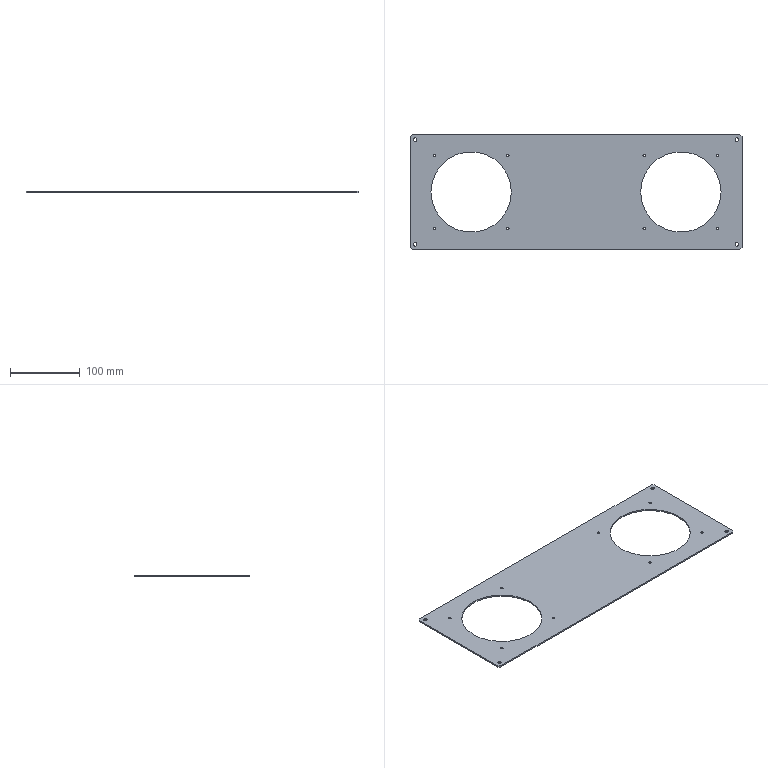Part | SolidWorks | features HoleWzd 2, Chamfer 1, Extrusion 1, ICE 1 | 1 solid | 38 faces | box 475 x 165 x 2 mm | volume 114873 mm3 | cylinder 28 | plane 10 | commonest cylinder face diameters 3.3 x16 5 x8 115 x4
STEP:
#1=CARTESIAN_POINT('',(-204.15,52.5,0.));
#2=VERTEX_POINT('',#1);
#3=CARTESIAN_POINT('',(-200.85,52.5,0.));
#4=VERTEX_POINT('',#3);
#5=CARTESIAN_POINT('',(-202.5,52.5,0.));
#6=DIRECTION('',(0.,0.,1.));
#7=DIRECTION('',(1.,0.,0.));
#8=AXIS2_PLACEMENT_3D('',#5,#6,#7);
#9=CIRCLE('',#8,1.65);
#10=EDGE_CURVE('',#2,#4,#9,.T.);
#11=ORIENTED_EDGE('',*,*,#10,.F.);
#12=CARTESIAN_POINT('',(-204.15,52.5,2.));
#13=VERTEX_POINT('',#12);
#14=CARTESIAN_POINT('',(-204.15,52.5,2.));
#15=DIRECTION('',(0.,0.,1.));
#16=VECTOR('',#15,1000.);
#17=LINE('',#14,#16);
#18=EDGE_CURVE('',#2,#13,#17,.T.);
#19=ORIENTED_EDGE('',*,*,#18,.T.);
#20=CARTESIAN_POINT('',(-200.85,52.5,2.));
#21=VERTEX_POINT('',#20);
#22=CARTESIAN_POINT('',(-202.5,52.5,2.));
#23=DIRECTION('',(0.,0.,1.));
#24=DIRECTION('',(1.,0.,0.));
#25=AXIS2_PLACEMENT_3D('',#22,#23,#24);
#26=CIRCLE('',#25,1.65);
#27=EDGE_CURVE('',#13,#21,#26,.T.);
#28=ORIENTED_EDGE('',*,*,#27,.T.);
#29=CARTESIAN_POINT('',(-200.85,52.5,2.));
#30=DIRECTION('',(0.,0.,1.));
#31=VECTOR('',#30,1000.);
#32=LINE('',#29,#31);
#33=EDGE_CURVE('',#4,#21,#32,.T.);
#34=ORIENTED_EDGE('',*,*,#33,.F.);
#35=EDGE_LOOP('',(#11,#19,#28,#34));
#36=FACE_OUTER_BOUND('',#35,.T.);
#37=CARTESIAN_POINT('',(-202.5,52.5,2.));
#38=DIRECTION('',(0.,0.,1.));
#39=DIRECTION('',(1.,0.,0.));
#40=AXIS2_PLACEMENT_3D('',#37,#38,#39);
#41=CYLINDRICAL_SURFACE('',#40,1.65);
#42=ADVANCED_FACE('',(#36),#41,.F.);
#43=CARTESIAN_POINT('',(-99.15,52.5,0.));
#44=VERTEX_POINT('',#43);
#45=CARTESIAN_POINT('',(-95.85,52.5,0.));
#46=VERTEX_POINT('',#45);
#47=CARTESIAN_POINT('',(-97.5,52.5,0.));
#48=DIRECTION('',(0.,0.,1.));
#49=DIRECTION('',(1.,0.,0.));
#50=AXIS2_PLACEMENT_3D('',#47,#48,#49);
#51=CIRCLE('',#50,1.65);
#52=EDGE_CURVE('',#44,#46,#51,.T.);
#53=ORIENTED_EDGE('',*,*,#52,.F.);
#54=CARTESIAN_POINT('',(-99.15,52.5,2.));
#55=VERTEX_POINT('',#54);
#56=CARTESIAN_POINT('',(-99.15,52.5,2.));
#57=DIRECTION('',(0.,0.,1.));
#58=VECTOR('',#57,1000.);
#59=LINE('',#56,#58);
#60=EDGE_CURVE('',#44,#55,#59,.T.);
#61=ORIENTED_EDGE('',*,*,#60,.T.);
#62=CARTESIAN_POINT('',(-95.85,52.5,2.));
#63=VERTEX_POINT('',#62);
#64=CARTESIAN_POINT('',(-97.5,52.5,2.));
#65=DIRECTION('',(0.,0.,1.));
#66=DIRECTION('',(1.,0.,0.));
#67=AXIS2_PLACEMENT_3D('',#64,#65,#66);
#68=CIRCLE('',#67,1.65);
#69=EDGE_CURVE('',#55,#63,#68,.T.);
#70=ORIENTED_EDGE('',*,*,#69,.T.);
#71=CARTESIAN_POINT('',(-95.85,52.5,2.));
#72=DIRECTION('',(0.,0.,1.));
#73=VECTOR('',#72,1000.);
#74=LINE('',#71,#73);
#75=EDGE_CURVE('',#46,#63,#74,.T.);
#76=ORIENTED_EDGE('',*,*,#75,.F.);
#77=EDGE_LOOP('',(#53,#61,#70,#76));
#78=FACE_OUTER_BOUND('',#77,.T.);
#79=CARTESIAN_POINT('',(-97.5,52.5,2.));
#80=DIRECTION('',(0.,0.,1.));
#81=DIRECTION('',(1.,0.,0.));
#82=AXIS2_PLACEMENT_3D('',#79,#80,#81);
#83=CYLINDRICAL_SURFACE('',#82,1.65);
#84=ADVANCED_FACE('',(#78),#83,.F.);
#85=CARTESIAN_POINT('',(-99.15,-52.5,0.));
#86=VERTEX_POINT('',#85);
#87=CARTESIAN_POINT('',(-95.85,-52.5,0.));
#88=VERTEX_POINT('',#87);
#89=CARTESIAN_POINT('',(-97.5,-52.5,0.));
#90=DIRECTION('',(0.,0.,1.));
#91=DIRECTION('',(1.,0.,0.));
#92=AXIS2_PLACEMENT_3D('',#89,#90,#91);
#93=CIRCLE('',#92,1.65);
#94=EDGE_CURVE('',#86,#88,#93,.T.);
#95=ORIENTED_EDGE('',*,*,#94,.F.);
#96=CARTESIAN_POINT('',(-99.15,-52.5,2.));
#97=VERTEX_POINT('',#96);
#98=CARTESIAN_POINT('',(-99.15,-52.5,2.));
#99=DIRECTION('',(0.,0.,1.));
#100=VECTOR('',#99,1000.);
#101=LINE('',#98,#100);
#102=EDGE_CURVE('',#86,#97,#101,.T.);
#103=ORIENTED_EDGE('',*,*,#102,.T.);
#104=CARTESIAN_POINT('',(-95.85,-52.5,2.));
#105=VERTEX_POINT('',#104);
#106=CARTESIAN_POINT('',(-97.5,-52.5,2.));
#107=DIRECTION('',(0.,0.,1.));
#108=DIRECTION('',(1.,0.,0.));
#109=AXIS2_PLACEMENT_3D('',#106,#107,#108);
#110=CIRCLE('',#109,1.65);
#111=EDGE_CURVE('',#97,#105,#110,.T.);
#112=ORIENTED_EDGE('',*,*,#111,.T.);
#113=CARTESIAN_POINT('',(-95.85,-52.5,2.));
#114=DIRECTION('',(0.,0.,1.));
#115=VECTOR('',#114,1000.);
#116=LINE('',#113,#115);
#117=EDGE_CURVE('',#88,#105,#116,.T.);
#118=ORIENTED_EDGE('',*,*,#117,.F.);
#119=EDGE_LOOP('',(#95,#103,#112,#118));
#120=FACE_OUTER_BOUND('',#119,.T.);
#121=CARTESIAN_POINT('',(-97.5,-52.5,2.));
#122=DIRECTION('',(0.,0.,1.));
#123=DIRECTION('',(1.,0.,0.));
#124=AXIS2_PLACEMENT_3D('',#121,#122,#123);
#125=CYLINDRICAL_SURFACE('',#124,1.65);
#126=ADVANCED_FACE('',(#120),#125,.F.);
#127=CARTESIAN_POINT('',(-204.15,-52.5,0.));
#128=VERTEX_POINT('',#127);
#129=CARTESIAN_POINT('',(-200.85,-52.5,0.));
#130=VERTEX_POINT('',#129);
#131=CARTESIAN_POINT('',(-202.5,-52.5,0.));
#132=DIRECTION('',(0.,0.,1.));
#133=DIRECTION('',(1.,0.,0.));
#134=AXIS2_PLACEMENT_3D('',#131,#132,#133);
#135=CIRCLE('',#134,1.65);
#136=EDGE_CURVE('',#128,#130,#135,.T.);
#137=ORIENTED_EDGE('',*,*,#136,.F.);
#138=CARTESIAN_POINT('',(-204.15,-52.5,2.));
#139=VERTEX_POINT('',#138);
#140=CARTESIAN_POINT('',(-204.15,-52.5,2.));
#141=DIRECTION('',(0.,0.,1.));
#142=VECTOR('',#141,1000.);
#143=LINE('',#140,#142);
#144=EDGE_CURVE('',#128,#139,#143,.T.);
#145=ORIENTED_EDGE('',*,*,#144,.T.);
#146=CARTESIAN_POINT('',(-200.85,-52.5,2.));
#147=VERTEX_POINT('',#146);
#148=CARTESIAN_POINT('',(-202.5,-52.5,2.));
#149=DIRECTION('',(0.,0.,1.));
#150=DIRECTION('',(1.,0.,0.));
#151=AXIS2_PLACEMENT_3D('',#148,#149,#150);
#152=CIRCLE('',#151,1.65);
#153=EDGE_CURVE('',#139,#147,#152,.T.);
#154=ORIENTED_EDGE('',*,*,#153,.T.);
#155=CARTESIAN_POINT('',(-200.85,-52.5,2.));
#156=DIRECTION('',(0.,0.,1.));
#157=VECTOR('',#156,1000.);
#158=LINE('',#155,#157);
#159=EDGE_CURVE('',#130,#147,#158,.T.);
#160=ORIENTED_EDGE('',*,*,#159,.F.);
#161=EDGE_LOOP('',(#137,#145,#154,#160));
#162=FACE_OUTER_BOUND('',#161,.T.);
#163=CARTESIAN_POINT('',(-202.5,-52.5,2.));
#164=DIRECTION('',(0.,0.,1.));
#165=DIRECTION('',(1.,0.,0.));
#166=AXIS2_PLACEMENT_3D('',#163,#164,#165);
#167=CYLINDRICAL_SURFACE('',#166,1.65);
#168=ADVANCED_FACE('',(#162),#167,.F.);
#169=CARTESIAN_POINT('',(95.85,-52.5,0.));
#170=VERTEX_POINT('',#169);
#171=CARTESIAN_POINT('',(99.15,-52.5,0.));
#172=VERTEX_POINT('',#171);
#173=CARTESIAN_POINT('',(97.5,-52.5,0.));
#174=DIRECTION('',(0.,0.,1.));
#175=DIRECTION('',(1.,0.,0.));
#176=AXIS2_PLACEMENT_3D('',#173,#174,#175);
#177=CIRCLE('',#176,1.65);
#178=EDGE_CURVE('',#170,#172,#177,.T.);
#179=ORIENTED_EDGE('',*,*,#178,.F.);
#180=CARTESIAN_POINT('',(95.85,-52.5,2.));
#181=VERTEX_POINT('',#180);
#182=CARTESIAN_POINT('',(95.85,-52.5,2.));
#183=DIRECTION('',(0.,0.,1.));
#184=VECTOR('',#183,1000.);
#185=LINE('',#182,#184);
#186=EDGE_CURVE('',#170,#181,#185,.T.);
#187=ORIENTED_EDGE('',*,*,#186,.T.);
#188=CARTESIAN_POINT('',(99.15,-52.5,2.));
#189=VERTEX_POINT('',#188);
#190=CARTESIAN_POINT('',(97.5,-52.5,2.));
#191=DIRECTION('',(0.,0.,1.));
#192=DIRECTION('',(1.,0.,0.));
#193=AXIS2_PLACEMENT_3D('',#190,#191,#192);
#194=CIRCLE('',#193,1.65);
#195=EDGE_CURVE('',#181,#189,#194,.T.);
#196=ORIENTED_EDGE('',*,*,#195,.T.);
#197=CARTESIAN_POINT('',(99.15,-52.5,2.));
#198=DIRECTION('',(0.,0.,1.));
#199=VECTOR('',#198,1000.);
#200=LINE('',#197,#199);
#201=EDGE_CURVE('',#172,#189,#200,.T.);
#202=ORIENTED_EDGE('',*,*,#201,.F.);
#203=EDGE_LOOP('',(#179,#187,#196,#202));
#204=FACE_OUTER_BOUND('',#203,.T.);
#205=CARTESIAN_POINT('',(97.5,-52.5,2.));
#206=DIRECTION('',(0.,0.,1.));
#207=DIRECTION('',(1.,0.,0.));
#208=AXIS2_PLACEMENT_3D('',#205,#206,#207);
#209=CYLINDRICAL_SURFACE('',#208,1.65);
#210=ADVANCED_FACE('',(#204),#209,.F.);
#211=CARTESIAN_POINT('',(200.85,-52.5,0.));
#212=VERTEX_POINT('',#211);
#213=CARTESIAN_POINT('',(204.15,-52.5,0.));
#214=VERTEX_POINT('',#213);
#215=CARTESIAN_POINT('',(202.5,-52.5,0.));
#216=DIRECTION('',(0.,0.,1.));
#217=DIRECTION('',(1.,0.,0.));
#218=AXIS2_PLACEMENT_3D('',#215,#216,#217);
#219=CIRCLE('',#218,1.65);
#220=EDGE_CURVE('',#212,#214,#219,.T.);
#221=ORIENTED_EDGE('',*,*,#220,.F.);
#222=CARTESIAN_POINT('',(200.85,-52.5,2.));
#223=VERTEX_POINT('',#222);
#224=CARTESIAN_POINT('',(200.85,-52.5,2.));
#225=DIRECTION('',(0.,0.,1.));
#226=VECTOR('',#225,1000.);
#227=LINE('',#224,#226);
#228=EDGE_CURVE('',#212,#223,#227,.T.);
#229=ORIENTED_EDGE('',*,*,#228,.T.);
#230=CARTESIAN_POINT('',(204.15,-52.5,2.));
#231=VERTEX_POINT('',#230);
#232=CARTESIAN_POINT('',(202.5,-52.5,2.));
#233=DIRECTION('',(0.,0.,1.));
#234=DIRECTION('',(1.,0.,0.));
#235=AXIS2_PLACEMENT_3D('',#232,#233,#234);
#236=CIRCLE('',#235,1.65);
#237=EDGE_CURVE('',#223,#231,#236,.T.);
#238=ORIENTED_EDGE('',*,*,#237,.T.);
#239=CARTESIAN_POINT('',(204.15,-52.5,2.));
#240=DIRECTION('',(0.,0.,1.));
#241=VECTOR('',#240,1000.);
#242=LINE('',#239,#241);
#243=EDGE_CURVE('',#214,#231,#242,.T.);
#244=ORIENTED_EDGE('',*,*,#243,.F.);
#245=EDGE_LOOP('',(#221,#229,#238,#244));
#246=FACE_OUTER_BOUND('',#245,.T.);
#247=CARTESIAN_POINT('',(202.5,-52.5,2.));
#248=DIRECTION('',(0.,0.,1.));
#249=DIRECTION('',(1.,0.,0.));
#250=AXIS2_PLACEMENT_3D('',#247,#248,#249);
#251=CYLINDRICAL_SURFACE('',#250,1.65);
#252=ADVANCED_FACE('',(#246),#251,.F.);
#253=CARTESIAN_POINT('',(200.85,52.5,0.));
#254=VERTEX_POINT('',#253);
#255=CARTESIAN_POINT('',(204.15,52.5,0.));
#256=VERTEX_POINT('',#255);
#257=CARTESIAN_POINT('',(202.5,52.5,0.));
#258=DIRECTION('',(0.,0.,1.));
#259=DIRECTION('',(1.,0.,0.));
#260=AXIS2_PLACEMENT_3D('',#257,#258,#259);
#261=CIRCLE('',#260,1.65);
#262=EDGE_CURVE('',#254,#256,#261,.T.);
#263=ORIENTED_EDGE('',*,*,#262,.F.);
#264=CARTESIAN_POINT('',(200.85,52.5,2.));
#265=VERTEX_POINT('',#264);
#266=CARTESIAN_POINT('',(200.85,52.5,2.));
#267=DIRECTION('',(0.,0.,1.));
#268=VECTOR('',#267,1000.);
#269=LINE('',#266,#268);
#270=EDGE_CURVE('',#254,#265,#269,.T.);
#271=ORIENTED_EDGE('',*,*,#270,.T.);
#272=CARTESIAN_POINT('',(204.15,52.5,2.));
#273=VERTEX_POINT('',#272);
#274=CARTESIAN_POINT('',(202.5,52.5,2.));
#275=DIRECTION('',(0.,0.,1.));
#276=DIRECTION('',(1.,0.,0.));
#277=AXIS2_PLACEMENT_3D('',#274,#275,#276);
#278=CIRCLE('',#277,1.65);
#279=EDGE_CURVE('',#265,#273,#278,.T.);
#280=ORIENTED_EDGE('',*,*,#279,.T.);
#281=CARTESIAN_POINT('',(204.15,52.5,2.));
#282=DIRECTION('',(0.,0.,1.));
#283=VECTOR('',#282,1000.);
#284=LINE('',#281,#283);
#285=EDGE_CURVE('',#256,#273,#284,.T.);
#286=ORIENTED_EDGE('',*,*,#285,.F.);
#287=EDGE_LOOP('',(#263,#271,#280,#286));
#288=FACE_OUTER_BOUND('',#287,.T.);
#289=CARTESIAN_POINT('',(202.5,52.5,2.));
#290=DIRECTION('',(0.,0.,1.));
#291=DIRECTION('',(1.,0.,0.));
#292=AXIS2_PLACEMENT_3D('',#289,#290,#291);
#293=CYLINDRICAL_SURFACE('',#292,1.65);
#294=ADVANCED_FACE('',(#288),#293,.F.);
#295=CARTESIAN_POINT('',(95.85,52.5,0.));
#296=VERTEX_POINT('',#295);
#297=CARTESIAN_POINT('',(99.15,52.5,0.));
#298=VERTEX_POINT('',#297);
#299=CARTESIAN_POINT('',(97.5,52.5,0.));
#300=DIRECTION('',(0.,0.,1.));
#301=DIRECTION('',(1.,0.,0.));
#302=AXIS2_PLACEMENT_3D('',#299,#300,#301);
#303=CIRCLE('',#302,1.65);
#304=EDGE_CURVE('',#296,#298,#303,.T.);
#305=ORIENTED_EDGE('',*,*,#304,.F.);
#306=CARTESIAN_POINT('',(95.85,52.5,2.));
#307=VERTEX_POINT('',#306);
#308=CARTESIAN_POINT('',(95.85,52.5,2.));
#309=DIRECTION('',(0.,0.,1.));
#310=VECTOR('',#309,1000.);
#311=LINE('',#308,#310);
#312=EDGE_CURVE('',#296,#307,#311,.T.);
#313=ORIENTED_EDGE('',*,*,#312,.T.);
#314=CARTESIAN_POINT('',(99.15,52.5,2.));
#315=VERTEX_POINT('',#314);
#316=CARTESIAN_POINT('',(97.5,52.5,2.));
#317=DIRECTION('',(0.,0.,1.));
#318=DIRECTION('',(1.,0.,0.));
#319=AXIS2_PLACEMENT_3D('',#316,#317,#318);
#320=CIRCLE('',#319,1.65);
#321=EDGE_CURVE('',#307,#315,#320,.T.);
#322=ORIENTED_EDGE('',*,*,#321,.T.);
#323=CARTESIAN_POINT('',(99.15,52.5,2.));
#324=DIRECTION('',(0.,0.,1.));
#325=VECTOR('',#324,1000.);
#326=LINE('',#323,#325);
#327=EDGE_CURVE('',#298,#315,#326,.T.);
#328=ORIENTED_EDGE('',*,*,#327,.F.);
#329=EDGE_LOOP('',(#305,#313,#322,#328));
#330=FACE_OUTER_BOUND('',#329,.T.);
#331=CARTESIAN_POINT('',(97.5,52.5,2.));
#332=DIRECTION('',(0.,0.,1.));
#333=DIRECTION('',(1.,0.,0.));
#334=AXIS2_PLACEMENT_3D('',#331,#332,#333);
#335=CYLINDRICAL_SURFACE('',#334,1.65);
#336=ADVANCED_FACE('',(#330),#335,.F.);
#337=CARTESIAN_POINT('',(92.5,0.,0.));
#338=VERTEX_POINT('',#337);
#339=CARTESIAN_POINT('',(207.5,0.,0.));
#340=VERTEX_POINT('',#339);
#341=CARTESIAN_POINT('',(150.,0.,0.));
#342=DIRECTION('',(0.,0.,1.));
#343=DIRECTION('',(1.,0.,0.));
#344=AXIS2_PLACEMENT_3D('',#341,#342,#343);
#345=CIRCLE('',#344,57.5);
#346=EDGE_CURVE('',#338,#340,#345,.T.);
#347=ORIENTED_EDGE('',*,*,#346,.F.);
#348=CARTESIAN_POINT('',(92.5,0.,2.));
#349=VERTEX_POINT('',#348);
#350=CARTESIAN_POINT('',(92.5,0.,0.));
#351=DIRECTION('',(0.,0.,1.));
#352=VECTOR('',#351,1000.);
#353=LINE('',#350,#352);
#354=EDGE_CURVE('',#338,#349,#353,.T.);
#355=ORIENTED_EDGE('',*,*,#354,.T.);
#356=CARTESIAN_POINT('',(207.5,0.,2.));
#357=VERTEX_POINT('',#356);
#358=CARTESIAN_POINT('',(150.,0.,2.));
#359=DIRECTION('',(0.,0.,1.));
#360=DIRECTION('',(1.,0.,0.));
#361=AXIS2_PLACEMENT_3D('',#358,#359,#360);
#362=CIRCLE('',#361,57.5);
#363=EDGE_CURVE('',#349,#357,#362,.T.);
#364=ORIENTED_EDGE('',*,*,#363,.T.);
#365=CARTESIAN_POINT('',(207.5,0.,0.));
#366=DIRECTION('',(0.,0.,1.));
#367=VECTOR('',#366,1000.);
#368=LINE('',#365,#367);
#369=EDGE_CURVE('',#340,#357,#368,.T.);
#370=ORIENTED_EDGE('',*,*,#369,.F.);
#371=EDGE_LOOP('',(#347,#355,#364,#370));
#372=FACE_OUTER_BOUND('',#371,.T.);
#373=CARTESIAN_POINT('',(150.,0.,0.));
#374=DIRECTION('',(0.,0.,1.));
#375=DIRECTION('',(1.,0.,0.));
#376=AXIS2_PLACEMENT_3D('',#373,#374,#375);
#377=CYLINDRICAL_SURFACE('',#376,57.5);
#378=ADVANCED_FACE('',(#372),#377,.F.);
#379=CARTESIAN_POINT('',(-207.5,0.,0.));
#380=VERTEX_POINT('',#379);
#381=CARTESIAN_POINT('',(-92.5,0.,0.));
#382=VERTEX_POINT('',#381);
#383=CARTESIAN_POINT('',(-150.,0.,0.));
#384=DIRECTION('',(0.,0.,1.));
#385=DIRECTION('',(1.,0.,0.));
#386=AXIS2_PLACEMENT_3D('',#383,#384,#385);
#387=CIRCLE('',#386,57.5);
#388=EDGE_CURVE('',#380,#382,#387,.T.);
#389=ORIENTED_EDGE('',*,*,#388,.F.);
#390=CARTESIAN_POINT('',(-207.5,0.,2.));
#391=VERTEX_POINT('',#390);
#392=CARTESIAN_POINT('',(-207.5,0.,0.));
#393=DIRECTION('',(0.,0.,1.));
#394=VECTOR('',#393,1000.);
#395=LINE('',#392,#394);
#396=EDGE_CURVE('',#380,#391,#395,.T.);
#397=ORIENTED_EDGE('',*,*,#396,.T.);
#398=CARTESIAN_POINT('',(-92.5,0.,2.));
#399=VERTEX_POINT('',#398);
#400=CARTESIAN_POINT('',(-150.,0.,2.));
#401=DIRECTION('',(0.,0.,1.));
#402=DIRECTION('',(1.,0.,0.));
#403=AXIS2_PLACEMENT_3D('',#400,#401,#402);
#404=CIRCLE('',#403,57.5);
#405=EDGE_CURVE('',#391,#399,#404,.T.);
#406=ORIENTED_EDGE('',*,*,#405,.T.);
#407=CARTESIAN_POINT('',(-92.5,0.,0.));
#408=DIRECTION('',(0.,0.,1.));
#409=VECTOR('',#408,1000.);
#410=LINE('',#407,#409);
#411=EDGE_CURVE('',#382,#399,#410,.T.);
#412=ORIENTED_EDGE('',*,*,#411,.F.);
#413=EDGE_LOOP('',(#389,#397,#406,#412));
#414=FACE_OUTER_BOUND('',#413,.T.);
#415=CARTESIAN_POINT('',(-150.,0.,0.));
#416=DIRECTION('',(0.,0.,1.));
#417=DIRECTION('',(1.,0.,0.));
#418=AXIS2_PLACEMENT_3D('',#415,#416,#417);
#419=CYLINDRICAL_SURFACE('',#418,57.5);
#420=ADVANCED_FACE('',(#414),#419,.F.);
#421=CARTESIAN_POINT('',(-232.5,75.,0.));
#422=VERTEX_POINT('',#421);
#423=CARTESIAN_POINT('',(-227.5,75.,0.));
#424=VERTEX_POINT('',#423);
#425=CARTESIAN_POINT('',(-230.,75.,0.));
#426=DIRECTION('',(0.,0.,1.));
#427=DIRECTION('',(1.,0.,0.));
#428=AXIS2_PLACEMENT_3D('',#425,#426,#427);
#429=CIRCLE('',#428,2.5);
#430=EDGE_CURVE('',#422,#424,#429,.T.);
#431=ORIENTED_EDGE('',*,*,#430,.F.);
#432=CARTESIAN_POINT('',(-232.5,75.,2.));
#433=VERTEX_POINT('',#432);
#434=CARTESIAN_POINT('',(-232.5,75.,2.));
#435=DIRECTION('',(0.,0.,1.));
#436=VECTOR('',#435,1000.);
#437=LINE('',#434,#436);
#438=EDGE_CURVE('',#422,#433,#437,.T.);
#439=ORIENTED_EDGE('',*,*,#438,.T.);
#440=CARTESIAN_POINT('',(-227.5,75.,2.));
#441=VERTEX_POINT('',#440);
#442=CARTESIAN_POINT('',(-230.,75.,2.));
#443=DIRECTION('',(0.,0.,1.));
#444=DIRECTION('',(1.,0.,0.));
#445=AXIS2_PLACEMENT_3D('',#442,#443,#444);
#446=CIRCLE('',#445,2.5);
#447=EDGE_CURVE('',#433,#441,#446,.T.);
#448=ORIENTED_EDGE('',*,*,#447,.T.);
#449=CARTESIAN_POINT('',(-227.5,75.,2.));
#450=DIRECTION('',(0.,0.,1.));
#451=VECTOR('',#450,1000.);
#452=LINE('',#449,#451);
#453=EDGE_CURVE('',#424,#441,#452,.T.);
#454=ORIENTED_EDGE('',*,*,#453,.F.);
#455=EDGE_LOOP('',(#431,#439,#448,#454));
#456=FACE_OUTER_BOUND('',#455,.T.);
#457=CARTESIAN_POINT('',(-230.,75.,2.));
#458=DIRECTION('',(0.,0.,1.));
#459=DIRECTION('',(1.,0.,0.));
#460=AXIS2_PLACEMENT_3D('',#457,#458,#459);
#461=CYLINDRICAL_SURFACE('',#460,2.5);
#462=ADVANCED_FACE('',(#456),#461,.F.);
#463=CARTESIAN_POINT('',(-232.5,-75.,0.));
#464=VERTEX_POINT('',#463);
#465=CARTESIAN_POINT('',(-227.5,-75.,0.));
#466=VERTEX_POINT('',#465);
#467=CARTESIAN_POINT('',(-230.,-75.,0.));
#468=DIRECTION('',(0.,0.,1.));
#469=DIRECTION('',(1.,0.,0.));
#470=AXIS2_PLACEMENT_3D('',#467,#468,#469);
#471=CIRCLE('',#470,2.5);
#472=EDGE_CURVE('',#464,#466,#471,.T.);
#473=ORIENTED_EDGE('',*,*,#472,.F.);
#474=CARTESIAN_POINT('',(-232.5,-75.,2.));
#475=VERTEX_POINT('',#474);
#476=CARTESIAN_POINT('',(-232.5,-75.,2.));
#477=DIRECTION('',(0.,0.,1.));
#478=VECTOR('',#477,1000.);
#479=LINE('',#476,#478);
#480=EDGE_CURVE('',#464,#475,#479,.T.);
#481=ORIENTED_EDGE('',*,*,#480,.T.);
#482=CARTESIAN_POINT('',(-227.5,-75.,2.));
#483=VERTEX_POINT('',#482);
#484=CARTESIAN_POINT('',(-230.,-75.,2.));
#485=DIRECTION('',(0.,0.,1.));
#486=DIRECTION('',(1.,0.,0.));
#487=AXIS2_PLACEMENT_3D('',#484,#485,#486);
#488=CIRCLE('',#487,2.5);
#489=EDGE_CURVE('',#475,#483,#488,.T.);
#490=ORIENTED_EDGE('',*,*,#489,.T.);
#491=CARTESIAN_POINT('',(-227.5,-75.,2.));
#492=DIRECTION('',(0.,0.,1.));
#493=VECTOR('',#492,1000.);
#494=LINE('',#491,#493);
#495=EDGE_CURVE('',#466,#483,#494,.T.);
#496=ORIENTED_EDGE('',*,*,#495,.F.);
#497=EDGE_LOOP('',(#473,#481,#490,#496));
#498=FACE_OUTER_BOUND('',#497,.T.);
#499=CARTESIAN_POINT('',(-230.,-75.,2.));
#500=DIRECTION('',(0.,0.,1.));
#501=DIRECTION('',(1.,0.,0.));
#502=AXIS2_PLACEMENT_3D('',#499,#500,#501);
#503=CYLINDRICAL_SURFACE('',#502,2.5);
#504=ADVANCED_FACE('',(#498),#503,.F.);
#505=CARTESIAN_POINT('',(227.5,75.,0.));
#506=VERTEX_POINT('',#505);
#507=CARTESIAN_POINT('',(232.5,75.,0.));
#508=VERTEX_POINT('',#507);
#509=CARTESIAN_POINT('',(230.,75.,0.));
#510=DIRECTION('',(0.,0.,1.));
#511=DIRECTION('',(1.,0.,0.));
#512=AXIS2_PLACEMENT_3D('',#509,#510,#511);
#513=CIRCLE('',#512,2.5);
#514=EDGE_CURVE('',#506,#508,#513,.T.);
#515=ORIENTED_EDGE('',*,*,#514,.F.);
#516=CARTESIAN_POINT('',(227.5,75.,2.));
#517=VERTEX_POINT('',#516);
#518=CARTESIAN_POINT('',(227.5,75.,2.));
#519=DIRECTION('',(0.,0.,1.));
#520=VECTOR('',#519,1000.);
#521=LINE('',#518,#520);
#522=EDGE_CURVE('',#506,#517,#521,.T.);
#523=ORIENTED_EDGE('',*,*,#522,.T.);
#524=CARTESIAN_POINT('',(232.5,75.,2.));
#525=VERTEX_POINT('',#524);
#526=CARTESIAN_POINT('',(230.,75.,2.));
#527=DIRECTION('',(0.,0.,1.));
#528=DIRECTION('',(1.,0.,0.));
#529=AXIS2_PLACEMENT_3D('',#526,#527,#528);
#530=CIRCLE('',#529,2.5);
#531=EDGE_CURVE('',#517,#525,#530,.T.);
#532=ORIENTED_EDGE('',*,*,#531,.T.);
#533=CARTESIAN_POINT('',(232.5,75.,2.));
#534=DIRECTION('',(0.,0.,1.));
#535=VECTOR('',#534,1000.);
#536=LINE('',#533,#535);
#537=EDGE_CURVE('',#508,#525,#536,.T.);
#538=ORIENTED_EDGE('',*,*,#537,.F.);
#539=EDGE_LOOP('',(#515,#523,#532,#538));
#540=FACE_OUTER_BOUND('',#539,.T.);
#541=CARTESIAN_POINT('',(230.,75.,2.));
#542=DIRECTION('',(0.,0.,1.));
#543=DIRECTION('',(1.,0.,0.));
#544=AXIS2_PLACEMENT_3D('',#541,#542,#543);
#545=CYLINDRICAL_SURFACE('',#544,2.5);
#546=ADVANCED_FACE('',(#540),#545,.F.);
#547=CARTESIAN_POINT('',(227.5,-75.,0.));
#548=VERTEX_POINT('',#547);
#549=CARTESIAN_POINT('',(232.5,-75.,0.));
#550=VERTEX_POINT('',#549);
#551=CARTESIAN_POINT('',(230.,-75.,0.));
#552=DIRECTION('',(0.,0.,1.));
#553=DIRECTION('',(1.,0.,0.));
#554=AXIS2_PLACEMENT_3D('',#551,#552,#553);
#555=CIRCLE('',#554,2.5);
#556=EDGE_CURVE('',#548,#550,#555,.T.);
#557=ORIENTED_EDGE('',*,*,#556,.F.);
#558=CARTESIAN_POINT('',(227.5,-75.,2.));
#559=VERTEX_POINT('',#558);
#560=CARTESIAN_POINT('',(227.5,-75.,2.));
#561=DIRECTION('',(0.,0.,1.));
#562=VECTOR('',#561,1000.);
#563=LINE('',#560,#562);
#564=EDGE_CURVE('',#548,#559,#563,.T.);
#565=ORIENTED_EDGE('',*,*,#564,.T.);
#566=CARTESIAN_POINT('',(232.5,-75.,2.));
#567=VERTEX_POINT('',#566);
#568=CARTESIAN_POINT('',(230.,-75.,2.));
#569=DIRECTION('',(0.,0.,1.));
#570=DIRECTION('',(1.,0.,0.));
#571=AXIS2_PLACEMENT_3D('',#568,#569,#570);
#572=CIRCLE('',#571,2.5);
#573=EDGE_CURVE('',#559,#567,#572,.T.);
#574=ORIENTED_EDGE('',*,*,#573,.T.);
#575=CARTESIAN_POINT('',(232.5,-75.,2.));
#576=DIRECTION('',(0.,0.,1.));
#577=VECTOR('',#576,1000.);
#578=LINE('',#575,#577);
#579=EDGE_CURVE('',#550,#567,#578,.T.);
#580=ORIENTED_EDGE('',*,*,#579,.F.);
#581=EDGE_LOOP('',(#557,#565,#574,#580));
#582=FACE_OUTER_BOUND('',#581,.T.);
#583=CARTESIAN_POINT('',(230.,-75.,2.));
#584=DIRECTION('',(0.,0.,1.));
#585=DIRECTION('',(1.,0.,0.));
#586=AXIS2_PLACEMENT_3D('',#583,#584,#585);
#587=CYLINDRICAL_SURFACE('',#586,2.5);
#588=ADVANCED_FACE('',(#582),#587,.F.);
#589=CARTESIAN_POINT('',(237.5,-79.5,0.));
#590=VERTEX_POINT('',#589);
#591=CARTESIAN_POINT('',(237.5,79.5,0.));
#592=VERTEX_POINT('',#591);
#593=CARTESIAN_POINT('',(237.5,82.5,0.));
#594=DIRECTION('',(0.,1.,0.));
#595=VECTOR('',#594,1000.);
#596=LINE('',#593,#595);
#597=EDGE_CURVE('',#590,#592,#596,.T.);
#598=ORIENTED_EDGE('',*,*,#597,.T.);
#599=CARTESIAN_POINT('',(237.5,79.5,2.));
#600=VERTEX_POINT('',#599);
#601=CARTESIAN_POINT('',(237.5,79.5,2.));
#602=DIRECTION('',(0.,0.,1.));
#603=VECTOR('',#602,1000.);
#604=LINE('',#601,#603);
#605=EDGE_CURVE('',#592,#600,#604,.T.);
#606=ORIENTED_EDGE('',*,*,#605,.T.);
#607=CARTESIAN_POINT('',(237.5,-79.5,2.));
#608=VERTEX_POINT('',#607);
#609=CARTESIAN_POINT('',(237.5,82.5,2.));
#610=DIRECTION('',(0.,1.,0.));
#611=VECTOR('',#610,1000.);
#612=LINE('',#609,#611);
#613=EDGE_CURVE('',#608,#600,#612,.T.);
#614=ORIENTED_EDGE('',*,*,#613,.F.);
#615=CARTESIAN_POINT('',(237.5,-79.5,2.));
#616=DIRECTION('',(0.,0.,-1.));
#617=VECTOR('',#616,1000.);
#618=LINE('',#615,#617);
#619=EDGE_CURVE('',#608,#590,#618,.T.);
#620=ORIENTED_EDGE('',*,*,#619,.T.);
#621=EDGE_LOOP('',(#598,#606,#614,#620));
#622=FACE_OUTER_BOUND('',#621,.T.);
#623=CARTESIAN_POINT('',(237.5,82.5,2.));
#624=DIRECTION('',(-1.,0.,0.));
#625=DIRECTION('',(0.,0.,1.));
#626=AXIS2_PLACEMENT_3D('',#623,#624,#625);
#627=PLANE('',#626);
#628=ADVANCED_FACE('',(#622),#627,.F.);
#629=CARTESIAN_POINT('',(234.5,82.5,2.));
#630=VERTEX_POINT('',#629);
#631=CARTESIAN_POINT('',(-234.5,82.5,2.));
#632=VERTEX_POINT('',#631);
#633=CARTESIAN_POINT('',(-237.5,82.5,2.));
#634=DIRECTION('',(-1.,0.,0.));
#635=VECTOR('',#634,1000.);
#636=LINE('',#633,#635);
#637=EDGE_CURVE('',#630,#632,#636,.T.);
#638=ORIENTED_EDGE('',*,*,#637,.F.);
#639=CARTESIAN_POINT('',(234.5,82.5,0.));
#640=VERTEX_POINT('',#639);
#641=CARTESIAN_POINT('',(234.5,82.5,2.));
#642=DIRECTION('',(0.,0.,-1.));
#643=VECTOR('',#642,1000.);
#644=LINE('',#641,#643);
#645=EDGE_CURVE('',#630,#640,#644,.T.);
#646=ORIENTED_EDGE('',*,*,#645,.T.);
#647=CARTESIAN_POINT('',(-234.5,82.5,0.));
#648=VERTEX_POINT('',#647);
#649=CARTESIAN_POINT('',(-237.5,82.5,0.));
#650=DIRECTION('',(-1.,0.,0.));
#651=VECTOR('',#650,1000.);
#652=LINE('',#649,#651);
#653=EDGE_CURVE('',#640,#648,#652,.T.);
#654=ORIENTED_EDGE('',*,*,#653,.T.);
#655=CARTESIAN_POINT('',(-234.5,82.5,2.));
#656=DIRECTION('',(0.,0.,1.));
#657=VECTOR('',#656,1000.);
#658=LINE('',#655,#657);
#659=EDGE_CURVE('',#648,#632,#658,.T.);
#660=ORIENTED_EDGE('',*,*,#659,.T.);
#661=EDGE_LOOP('',(#638,#646,#654,#660));
#662=FACE_OUTER_BOUND('',#661,.T.);
#663=CARTESIAN_POINT('',(-237.5,82.5,2.));
#664=DIRECTION('',(0.,-1.,0.));
#665=DIRECTION('',(0.,0.,-1.));
#666=AXIS2_PLACEMENT_3D('',#663,#664,#665);
#667=PLANE('',#666);
#668=ADVANCED_FACE('',(#662),#667,.F.);
#669=CARTESIAN_POINT('',(-237.5,79.5,0.));
#670=VERTEX_POINT('',#669);
#671=CARTESIAN_POINT('',(-237.5,-79.5,0.));
#672=VERTEX_POINT('',#671);
#673=CARTESIAN_POINT('',(-237.5,82.5,0.));
#674=DIRECTION('',(0.,-1.,0.));
#675=VECTOR('',#674,1000.);
#676=LINE('',#673,#675);
#677=EDGE_CURVE('',#670,#672,#676,.T.);
#678=ORIENTED_EDGE('',*,*,#677,.T.);
#679=CARTESIAN_POINT('',(-237.5,-79.5,2.));
#680=VERTEX_POINT('',#679);
#681=CARTESIAN_POINT('',(-237.5,-79.5,2.));
#682=DIRECTION('',(0.,0.,1.));
#683=VECTOR('',#682,1000.);
#684=LINE('',#681,#683);
#685=EDGE_CURVE('',#672,#680,#684,.T.);
#686=ORIENTED_EDGE('',*,*,#685,.T.);
#687=CARTESIAN_POINT('',(-237.5,79.5,2.));
#688=VERTEX_POINT('',#687);
#689=CARTESIAN_POINT('',(-237.5,82.5,2.));
#690=DIRECTION('',(0.,-1.,0.));
#691=VECTOR('',#690,1000.);
#692=LINE('',#689,#691);
#693=EDGE_CURVE('',#688,#680,#692,.T.);
#694=ORIENTED_EDGE('',*,*,#693,.F.);
#695=CARTESIAN_POINT('',(-237.5,79.5,2.));
#696=DIRECTION('',(0.,0.,-1.));
#697=VECTOR('',#696,1000.);
#698=LINE('',#695,#697);
#699=EDGE_CURVE('',#688,#670,#698,.T.);
#700=ORIENTED_EDGE('',*,*,#699,.T.);
#701=EDGE_LOOP('',(#678,#686,#694,#700));
#702=FACE_OUTER_BOUND('',#701,.T.);
#703=CARTESIAN_POINT('',(-237.5,82.5,2.));
#704=DIRECTION('',(1.,0.,0.));
#705=DIRECTION('',(0.,0.,-1.));
#706=AXIS2_PLACEMENT_3D('',#703,#704,#705);
#707=PLANE('',#706);
#708=ADVANCED_FACE('',(#702),#707,.F.);
#709=CARTESIAN_POINT('',(-234.5,-82.5,0.));
#710=VERTEX_POINT('',#709);
#711=CARTESIAN_POINT('',(234.5,-82.5,0.));
#712=VERTEX_POINT('',#711);
#713=CARTESIAN_POINT('',(-237.5,-82.5,0.));
#714=DIRECTION('',(1.,0.,0.));
#715=VECTOR('',#714,1000.);
#716=LINE('',#713,#715);
#717=EDGE_CURVE('',#710,#712,#716,.T.);
#718=ORIENTED_EDGE('',*,*,#717,.T.);
#719=CARTESIAN_POINT('',(234.5,-82.5,2.));
#720=VERTEX_POINT('',#719);
#721=CARTESIAN_POINT('',(234.5,-82.5,2.));
#722=DIRECTION('',(0.,0.,1.));
#723=VECTOR('',#722,1000.);
#724=LINE('',#721,#723);
#725=EDGE_CURVE('',#712,#720,#724,.T.);
#726=ORIENTED_EDGE('',*,*,#725,.T.);
#727=CARTESIAN_POINT('',(-234.5,-82.5,2.));
#728=VERTEX_POINT('',#727);
#729=CARTESIAN_POINT('',(-237.5,-82.5,2.));
#730=DIRECTION('',(1.,0.,0.));
#731=VECTOR('',#730,1000.);
#732=LINE('',#729,#731);
#733=EDGE_CURVE('',#728,#720,#732,.T.);
#734=ORIENTED_EDGE('',*,*,#733,.F.);
#735=CARTESIAN_POINT('',(-234.5,-82.5,2.));
#736=DIRECTION('',(0.,0.,-1.));
#737=VECTOR('',#736,1000.);
#738=LINE('',#735,#737);
#739=EDGE_CURVE('',#728,#710,#738,.T.);
#740=ORIENTED_EDGE('',*,*,#739,.T.);
#741=EDGE_LOOP('',(#718,#726,#734,#740));
#742=FACE_OUTER_BOUND('',#741,.T.);
#743=CARTESIAN_POINT('',(-237.5,-82.5,2.));
#744=DIRECTION('',(0.,1.,0.));
#745=DIRECTION('',(0.,0.,1.));
#746=AXIS2_PLACEMENT_3D('',#743,#744,#745);
#747=PLANE('',#746);
#748=ADVANCED_FACE('',(#742),#747,.F.);
#749=CARTESIAN_POINT('',(-202.5,52.5,2.));
#750=DIRECTION('',(0.,0.,1.));
#751=DIRECTION('',(1.,0.,0.));
#752=AXIS2_PLACEMENT_3D('',#749,#750,#751);
#753=CIRCLE('',#752,1.65);
#754=EDGE_CURVE('',#21,#13,#753,.T.);
#755=ORIENTED_EDGE('',*,*,#754,.F.);
#756=ORIENTED_EDGE('',*,*,#27,.F.);
#757=EDGE_LOOP('',(#755,#756));
#758=FACE_BOUND('',#757,.T.);
#759=CARTESIAN_POINT('',(-97.5,52.5,2.));
#760=DIRECTION('',(0.,0.,1.));
#761=DIRECTION('',(1.,0.,0.));
#762=AXIS2_PLACEMENT_3D('',#759,#760,#761);
#763=CIRCLE('',#762,1.65);
#764=EDGE_CURVE('',#63,#55,#763,.T.);
#765=ORIENTED_EDGE('',*,*,#764,.F.);
#766=ORIENTED_EDGE('',*,*,#69,.F.);
#767=EDGE_LOOP('',(#765,#766));
#768=FACE_BOUND('',#767,.T.);
#769=CARTESIAN_POINT('',(-97.5,-52.5,2.));
#770=DIRECTION('',(0.,0.,1.));
#771=DIRECTION('',(1.,0.,0.));
#772=AXIS2_PLACEMENT_3D('',#769,#770,#771);
#773=CIRCLE('',#772,1.65);
#774=EDGE_CURVE('',#105,#97,#773,.T.);
#775=ORIENTED_EDGE('',*,*,#774,.F.);
#776=ORIENTED_EDGE('',*,*,#111,.F.);
#777=EDGE_LOOP('',(#775,#776));
#778=FACE_BOUND('',#777,.T.);
#779=CARTESIAN_POINT('',(-202.5,-52.5,2.));
#780=DIRECTION('',(0.,0.,1.));
#781=DIRECTION('',(1.,0.,0.));
#782=AXIS2_PLACEMENT_3D('',#779,#780,#781);
#783=CIRCLE('',#782,1.65);
#784=EDGE_CURVE('',#147,#139,#783,.T.);
#785=ORIENTED_EDGE('',*,*,#784,.F.);
#786=ORIENTED_EDGE('',*,*,#153,.F.);
#787=EDGE_LOOP('',(#785,#786));
#788=FACE_BOUND('',#787,.T.);
#789=CARTESIAN_POINT('',(97.5,-52.5,2.));
#790=DIRECTION('',(0.,0.,1.));
#791=DIRECTION('',(1.,0.,0.));
#792=AXIS2_PLACEMENT_3D('',#789,#790,#791);
#793=CIRCLE('',#792,1.65);
#794=EDGE_CURVE('',#189,#181,#793,.T.);
#795=ORIENTED_EDGE('',*,*,#794,.F.);
#796=ORIENTED_EDGE('',*,*,#195,.F.);
#797=EDGE_LOOP('',(#795,#796));
#798=FACE_BOUND('',#797,.T.);
#799=CARTESIAN_POINT('',(202.5,-52.5,2.));
#800=DIRECTION('',(0.,0.,1.));
#801=DIRECTION('',(1.,0.,0.));
#802=AXIS2_PLACEMENT_3D('',#799,#800,#801);
#803=CIRCLE('',#802,1.65);
#804=EDGE_CURVE('',#231,#223,#803,.T.);
#805=ORIENTED_EDGE('',*,*,#804,.F.);
#806=ORIENTED_EDGE('',*,*,#237,.F.);
#807=EDGE_LOOP('',(#805,#806));
#808=FACE_BOUND('',#807,.T.);
#809=CARTESIAN_POINT('',(202.5,52.5,2.));
#810=DIRECTION('',(0.,0.,1.));
#811=DIRECTION('',(1.,0.,0.));
#812=AXIS2_PLACEMENT_3D('',#809,#810,#811);
#813=CIRCLE('',#812,1.65);
#814=EDGE_CURVE('',#273,#265,#813,.T.);
#815=ORIENTED_EDGE('',*,*,#814,.F.);
#816=ORIENTED_EDGE('',*,*,#279,.F.);
#817=EDGE_LOOP('',(#815,#816));
#818=FACE_BOUND('',#817,.T.);
#819=CARTESIAN_POINT('',(97.5,52.5,2.));
#820=DIRECTION('',(0.,0.,1.));
#821=DIRECTION('',(1.,0.,0.));
#822=AXIS2_PLACEMENT_3D('',#819,#820,#821);
#823=CIRCLE('',#822,1.65);
#824=EDGE_CURVE('',#315,#307,#823,.T.);
#825=ORIENTED_EDGE('',*,*,#824,.F.);
#826=ORIENTED_EDGE('',*,*,#321,.F.);
#827=EDGE_LOOP('',(#825,#826));
#828=FACE_BOUND('',#827,.T.);
#829=CARTESIAN_POINT('',(150.,0.,2.));
#830=DIRECTION('',(0.,0.,1.));
#831=DIRECTION('',(1.,0.,0.));
#832=AXIS2_PLACEMENT_3D('',#829,#830,#831);
#833=CIRCLE('',#832,57.5);
#834=EDGE_CURVE('',#357,#349,#833,.T.);
#835=ORIENTED_EDGE('',*,*,#834,.F.);
#836=ORIENTED_EDGE('',*,*,#363,.F.);
#837=EDGE_LOOP('',(#835,#836));
#838=FACE_BOUND('',#837,.T.);
#839=CARTESIAN_POINT('',(-150.,0.,2.));
#840=DIRECTION('',(0.,0.,1.));
#841=DIRECTION('',(1.,0.,0.));
#842=AXIS2_PLACEMENT_3D('',#839,#840,#841);
#843=CIRCLE('',#842,57.5);
#844=EDGE_CURVE('',#399,#391,#843,.T.);
#845=ORIENTED_EDGE('',*,*,#844,.F.);
#846=ORIENTED_EDGE('',*,*,#405,.F.);
#847=EDGE_LOOP('',(#845,#846));
#848=FACE_BOUND('',#847,.T.);
#849=CARTESIAN_POINT('',(-230.,75.,2.));
#850=DIRECTION('',(0.,0.,1.));
#851=DIRECTION('',(1.,0.,0.));
#852=AXIS2_PLACEMENT_3D('',#849,#850,#851);
#853=CIRCLE('',#852,2.5);
#854=EDGE_CURVE('',#441,#433,#853,.T.);
#855=ORIENTED_EDGE('',*,*,#854,.F.);
#856=ORIENTED_EDGE('',*,*,#447,.F.);
#857=EDGE_LOOP('',(#855,#856));
#858=FACE_BOUND('',#857,.T.);
#859=CARTESIAN_POINT('',(-230.,-75.,2.));
#860=DIRECTION('',(0.,0.,1.));
#861=DIRECTION('',(1.,0.,0.));
#862=AXIS2_PLACEMENT_3D('',#859,#860,#861);
#863=CIRCLE('',#862,2.5);
#864=EDGE_CURVE('',#483,#475,#863,.T.);
#865=ORIENTED_EDGE('',*,*,#864,.F.);
#866=ORIENTED_EDGE('',*,*,#489,.F.);
#867=EDGE_LOOP('',(#865,#866));
#868=FACE_BOUND('',#867,.T.);
#869=CARTESIAN_POINT('',(230.,75.,2.));
#870=DIRECTION('',(0.,0.,1.));
#871=DIRECTION('',(1.,0.,0.));
#872=AXIS2_PLACEMENT_3D('',#869,#870,#871);
#873=CIRCLE('',#872,2.5);
#874=EDGE_CURVE('',#525,#517,#873,.T.);
#875=ORIENTED_EDGE('',*,*,#874,.F.);
#876=ORIENTED_EDGE('',*,*,#531,.F.);
#877=EDGE_LOOP('',(#875,#876));
#878=FACE_BOUND('',#877,.T.);
#879=CARTESIAN_POINT('',(230.,-75.,2.));
#880=DIRECTION('',(0.,0.,1.));
#881=DIRECTION('',(1.,0.,0.));
#882=AXIS2_PLACEMENT_3D('',#879,#880,#881);
#883=CIRCLE('',#882,2.5);
#884=EDGE_CURVE('',#567,#559,#883,.T.);
#885=ORIENTED_EDGE('',*,*,#884,.F.);
#886=ORIENTED_EDGE('',*,*,#573,.F.);
#887=EDGE_LOOP('',(#885,#886));
#888=FACE_BOUND('',#887,.T.);
#889=ORIENTED_EDGE('',*,*,#613,.T.);
#890=CARTESIAN_POINT('',(158.5,158.5,2.));
#891=DIRECTION('',(-0.7071,0.7071,0.));
#892=VECTOR('',#891,1000.);
#893=LINE('',#890,#892);
#894=EDGE_CURVE('',#600,#630,#893,.T.);
#895=ORIENTED_EDGE('',*,*,#894,.T.);
#896=ORIENTED_EDGE('',*,*,#637,.T.);
#897=CARTESIAN_POINT('',(-158.5,158.5,2.));
#898=DIRECTION('',(-0.7071,-0.7071,0.));
#899=VECTOR('',#898,1000.);
#900=LINE('',#897,#899);
#901=EDGE_CURVE('',#632,#688,#900,.T.);
#902=ORIENTED_EDGE('',*,*,#901,.T.);
#903=ORIENTED_EDGE('',*,*,#693,.T.);
#904=CARTESIAN_POINT('',(-158.5,-158.5,2.));
#905=DIRECTION('',(0.7071,-0.7071,0.));
#906=VECTOR('',#905,1000.);
#907=LINE('',#904,#906);
#908=EDGE_CURVE('',#680,#728,#907,.T.);
#909=ORIENTED_EDGE('',*,*,#908,.T.);
#910=ORIENTED_EDGE('',*,*,#733,.T.);
#911=CARTESIAN_POINT('',(158.5,-158.5,2.));
#912=DIRECTION('',(0.7071,0.7071,0.));
#913=VECTOR('',#912,1000.);
#914=LINE('',#911,#913);
#915=EDGE_CURVE('',#720,#608,#914,.T.);
#916=ORIENTED_EDGE('',*,*,#915,.T.);
#917=EDGE_LOOP('',(#889,#895,#896,#902,#903,#909,#910,#916));
#918=FACE_OUTER_BOUND('',#917,.T.);
#919=CARTESIAN_POINT('',(0.,0.,2.));
#920=DIRECTION('',(0.,0.,1.));
#921=DIRECTION('',(1.,0.,0.));
#922=AXIS2_PLACEMENT_3D('',#919,#920,#921);
#923=PLANE('',#922);
#924=ADVANCED_FACE('',(#758,#768,#778,#788,#798,#808,#818,#828,#838,#848,#858,#868,#878,#888,#918),#923,.T.);
#925=CARTESIAN_POINT('',(-202.5,52.5,0.));
#926=DIRECTION('',(0.,0.,1.));
#927=DIRECTION('',(1.,0.,0.));
#928=AXIS2_PLACEMENT_3D('',#925,#926,#927);
#929=CIRCLE('',#928,1.65);
#930=EDGE_CURVE('',#4,#2,#929,.T.);
#931=ORIENTED_EDGE('',*,*,#930,.T.);
#932=ORIENTED_EDGE('',*,*,#10,.T.);
#933=EDGE_LOOP('',(#931,#932));
#934=FACE_BOUND('',#933,.T.);
#935=CARTESIAN_POINT('',(-97.5,52.5,0.));
#936=DIRECTION('',(0.,0.,1.));
#937=DIRECTION('',(1.,0.,0.));
#938=AXIS2_PLACEMENT_3D('',#935,#936,#937);
#939=CIRCLE('',#938,1.65);
#940=EDGE_CURVE('',#46,#44,#939,.T.);
#941=ORIENTED_EDGE('',*,*,#940,.T.);
#942=ORIENTED_EDGE('',*,*,#52,.T.);
#943=EDGE_LOOP('',(#941,#942));
#944=FACE_BOUND('',#943,.T.);
#945=CARTESIAN_POINT('',(-97.5,-52.5,0.));
#946=DIRECTION('',(0.,0.,1.));
#947=DIRECTION('',(1.,0.,0.));
#948=AXIS2_PLACEMENT_3D('',#945,#946,#947);
#949=CIRCLE('',#948,1.65);
#950=EDGE_CURVE('',#88,#86,#949,.T.);
#951=ORIENTED_EDGE('',*,*,#950,.T.);
#952=ORIENTED_EDGE('',*,*,#94,.T.);
#953=EDGE_LOOP('',(#951,#952));
#954=FACE_BOUND('',#953,.T.);
#955=CARTESIAN_POINT('',(-202.5,-52.5,0.));
#956=DIRECTION('',(0.,0.,1.));
#957=DIRECTION('',(1.,0.,0.));
#958=AXIS2_PLACEMENT_3D('',#955,#956,#957);
#959=CIRCLE('',#958,1.65);
#960=EDGE_CURVE('',#130,#128,#959,.T.);
#961=ORIENTED_EDGE('',*,*,#960,.T.);
#962=ORIENTED_EDGE('',*,*,#136,.T.);
#963=EDGE_LOOP('',(#961,#962));
#964=FACE_BOUND('',#963,.T.);
#965=CARTESIAN_POINT('',(97.5,-52.5,0.));
#966=DIRECTION('',(0.,0.,1.));
#967=DIRECTION('',(1.,0.,0.));
#968=AXIS2_PLACEMENT_3D('',#965,#966,#967);
#969=CIRCLE('',#968,1.65);
#970=EDGE_CURVE('',#172,#170,#969,.T.);
#971=ORIENTED_EDGE('',*,*,#970,.T.);
#972=ORIENTED_EDGE('',*,*,#178,.T.);
#973=EDGE_LOOP('',(#971,#972));
#974=FACE_BOUND('',#973,.T.);
#975=CARTESIAN_POINT('',(202.5,-52.5,0.));
#976=DIRECTION('',(0.,0.,1.));
#977=DIRECTION('',(1.,0.,0.));
#978=AXIS2_PLACEMENT_3D('',#975,#976,#977);
#979=CIRCLE('',#978,1.65);
#980=EDGE_CURVE('',#214,#212,#979,.T.);
#981=ORIENTED_EDGE('',*,*,#980,.T.);
#982=ORIENTED_EDGE('',*,*,#220,.T.);
#983=EDGE_LOOP('',(#981,#982));
#984=FACE_BOUND('',#983,.T.);
#985=CARTESIAN_POINT('',(202.5,52.5,0.));
#986=DIRECTION('',(0.,0.,1.));
#987=DIRECTION('',(1.,0.,0.));
#988=AXIS2_PLACEMENT_3D('',#985,#986,#987);
#989=CIRCLE('',#988,1.65);
#990=EDGE_CURVE('',#256,#254,#989,.T.);
#991=ORIENTED_EDGE('',*,*,#990,.T.);
#992=ORIENTED_EDGE('',*,*,#262,.T.);
#993=EDGE_LOOP('',(#991,#992));
#994=FACE_BOUND('',#993,.T.);
#995=CARTESIAN_POINT('',(97.5,52.5,0.));
#996=DIRECTION('',(0.,0.,1.));
#997=DIRECTION('',(1.,0.,0.));
#998=AXIS2_PLACEMENT_3D('',#995,#996,#997);
#999=CIRCLE('',#998,1.65);
#1000=EDGE_CURVE('',#298,#296,#999,.T.);
#1001=ORIENTED_EDGE('',*,*,#1000,.T.);
#1002=ORIENTED_EDGE('',*,*,#304,.T.);
#1003=EDGE_LOOP('',(#1001,#1002));
#1004=FACE_BOUND('',#1003,.T.);
#1005=CARTESIAN_POINT('',(150.,0.,0.));
#1006=DIRECTION('',(0.,0.,1.));
#1007=DIRECTION('',(1.,0.,0.));
#1008=AXIS2_PLACEMENT_3D('',#1005,#1006,#1007);
#1009=CIRCLE('',#1008,57.5);
#1010=EDGE_CURVE('',#340,#338,#1009,.T.);
#1011=ORIENTED_EDGE('',*,*,#1010,.T.);
#1012=ORIENTED_EDGE('',*,*,#346,.T.);
#1013=EDGE_LOOP('',(#1011,#1012));
#1014=FACE_BOUND('',#1013,.T.);
#1015=CARTESIAN_POINT('',(-150.,0.,0.));
#1016=DIRECTION('',(0.,0.,1.));
#1017=DIRECTION('',(1.,0.,0.));
#1018=AXIS2_PLACEMENT_3D('',#1015,#1016,#1017);
#1019=CIRCLE('',#1018,57.5);
#1020=EDGE_CURVE('',#382,#380,#1019,.T.);
#1021=ORIENTED_EDGE('',*,*,#1020,.T.);
#1022=ORIENTED_EDGE('',*,*,#388,.T.);
#1023=EDGE_LOOP('',(#1021,#1022));
#1024=FACE_BOUND('',#1023,.T.);
#1025=CARTESIAN_POINT('',(-230.,75.,0.));
#1026=DIRECTION('',(0.,0.,1.));
#1027=DIRECTION('',(1.,0.,0.));
#1028=AXIS2_PLACEMENT_3D('',#1025,#1026,#1027);
#1029=CIRCLE('',#1028,2.5);
#1030=EDGE_CURVE('',#424,#422,#1029,.T.);
#1031=ORIENTED_EDGE('',*,*,#1030,.T.);
#1032=ORIENTED_EDGE('',*,*,#430,.T.);
#1033=EDGE_LOOP('',(#1031,#1032));
#1034=FACE_BOUND('',#1033,.T.);
#1035=CARTESIAN_POINT('',(-230.,-75.,0.));
#1036=DIRECTION('',(0.,0.,1.));
#1037=DIRECTION('',(1.,0.,0.));
#1038=AXIS2_PLACEMENT_3D('',#1035,#1036,#1037);
#1039=CIRCLE('',#1038,2.5);
#1040=EDGE_CURVE('',#466,#464,#1039,.T.);
#1041=ORIENTED_EDGE('',*,*,#1040,.T.);
#1042=ORIENTED_EDGE('',*,*,#472,.T.);
#1043=EDGE_LOOP('',(#1041,#1042));
#1044=FACE_BOUND('',#1043,.T.);
#1045=CARTESIAN_POINT('',(230.,75.,0.));
#1046=DIRECTION('',(0.,0.,1.));
#1047=DIRECTION('',(1.,0.,0.));
#1048=AXIS2_PLACEMENT_3D('',#1045,#1046,#1047);
#1049=CIRCLE('',#1048,2.5);
#1050=EDGE_CURVE('',#508,#506,#1049,.T.);
#1051=ORIENTED_EDGE('',*,*,#1050,.T.);
#1052=ORIENTED_EDGE('',*,*,#514,.T.);
#1053=EDGE_LOOP('',(#1051,#1052));
#1054=FACE_BOUND('',#1053,.T.);
#1055=CARTESIAN_POINT('',(230.,-75.,0.));
#1056=DIRECTION('',(0.,0.,1.));
#1057=DIRECTION('',(1.,0.,0.));
#1058=AXIS2_PLACEMENT_3D('',#1055,#1056,#1057);
#1059=CIRCLE('',#1058,2.5);
#1060=EDGE_CURVE('',#550,#548,#1059,.T.);
#1061=ORIENTED_EDGE('',*,*,#1060,.T.);
#1062=ORIENTED_EDGE('',*,*,#556,.T.);
#1063=EDGE_LOOP('',(#1061,#1062));
#1064=FACE_BOUND('',#1063,.T.);
#1065=ORIENTED_EDGE('',*,*,#653,.F.);
#1066=CARTESIAN_POINT('',(234.5,82.5,0.));
#1067=DIRECTION('',(0.7071,-0.7071,0.));
#1068=VECTOR('',#1067,1000.);
#1069=LINE('',#1066,#1068);
#1070=EDGE_CURVE('',#640,#592,#1069,.T.);
#1071=ORIENTED_EDGE('',*,*,#1070,.T.);
#1072=ORIENTED_EDGE('',*,*,#597,.F.);
#1073=CARTESIAN_POINT('',(237.5,-79.5,0.));
#1074=DIRECTION('',(-0.7071,-0.7071,0.));
#1075=VECTOR('',#1074,1000.);
#1076=LINE('',#1073,#1075);
#1077=EDGE_CURVE('',#590,#712,#1076,.T.);
#1078=ORIENTED_EDGE('',*,*,#1077,.T.);
#1079=ORIENTED_EDGE('',*,*,#717,.F.);
#1080=CARTESIAN_POINT('',(-234.5,-82.5,0.));
#1081=DIRECTION('',(-0.7071,0.7071,0.));
#1082=VECTOR('',#1081,1000.);
#1083=LINE('',#1080,#1082);
#1084=EDGE_CURVE('',#710,#672,#1083,.T.);
#1085=ORIENTED_EDGE('',*,*,#1084,.T.);
#1086=ORIENTED_EDGE('',*,*,#677,.F.);
#1087=CARTESIAN_POINT('',(-237.5,79.5,0.));
#1088=DIRECTION('',(0.7071,0.7071,0.));
#1089=VECTOR('',#1088,1000.);
#1090=LINE('',#1087,#1089);
#1091=EDGE_CURVE('',#670,#648,#1090,.T.);
#1092=ORIENTED_EDGE('',*,*,#1091,.T.);
#1093=EDGE_LOOP('',(#1065,#1071,#1072,#1078,#1079,#1085,#1086,#1092));
#1094=FACE_OUTER_BOUND('',#1093,.T.);
#1095=CARTESIAN_POINT('',(0.,0.,0.));
#1096=DIRECTION('',(0.,0.,1.));
#1097=DIRECTION('',(1.,0.,0.));
#1098=AXIS2_PLACEMENT_3D('',#1095,#1096,#1097);
#1099=PLANE('',#1098);
#1100=ADVANCED_FACE('',(#934,#944,#954,#964,#974,#984,#994,#1004,#1014,#1024,#1034,#1044,#1054,#1064,#1094),#1099,.F.);
#1101=ORIENTED_EDGE('',*,*,#564,.F.);
#1102=ORIENTED_EDGE('',*,*,#1060,.F.);
#1103=ORIENTED_EDGE('',*,*,#579,.T.);
#1104=ORIENTED_EDGE('',*,*,#884,.T.);
#1105=EDGE_LOOP('',(#1101,#1102,#1103,#1104));
#1106=FACE_OUTER_BOUND('',#1105,.T.);
#1107=CARTESIAN_POINT('',(230.,-75.,2.));
#1108=DIRECTION('',(0.,0.,1.));
#1109=DIRECTION('',(1.,0.,0.));
#1110=AXIS2_PLACEMENT_3D('',#1107,#1108,#1109);
#1111=CYLINDRICAL_SURFACE('',#1110,2.5);
#1112=ADVANCED_FACE('',(#1106),#1111,.F.);
#1113=ORIENTED_EDGE('',*,*,#522,.F.);
#1114=ORIENTED_EDGE('',*,*,#1050,.F.);
#1115=ORIENTED_EDGE('',*,*,#537,.T.);
#1116=ORIENTED_EDGE('',*,*,#874,.T.);
#1117=EDGE_LOOP('',(#1113,#1114,#1115,#1116));
#1118=FACE_OUTER_BOUND('',#1117,.T.);
#1119=CARTESIAN_POINT('',(230.,75.,2.));
#1120=DIRECTION('',(0.,0.,1.));
#1121=DIRECTION('',(1.,0.,0.));
#1122=AXIS2_PLACEMENT_3D('',#1119,#1120,#1121);
#1123=CYLINDRICAL_SURFACE('',#1122,2.5);
#1124=ADVANCED_FACE('',(#1118),#1123,.F.);
#1125=ORIENTED_EDGE('',*,*,#480,.F.);
#1126=ORIENTED_EDGE('',*,*,#1040,.F.);
#1127=ORIENTED_EDGE('',*,*,#495,.T.);
#1128=ORIENTED_EDGE('',*,*,#864,.T.);
#1129=EDGE_LOOP('',(#1125,#1126,#1127,#1128));
#1130=FACE_OUTER_BOUND('',#1129,.T.);
#1131=CARTESIAN_POINT('',(-230.,-75.,2.));
#1132=DIRECTION('',(0.,0.,1.));
#1133=DIRECTION('',(1.,0.,0.));
#1134=AXIS2_PLACEMENT_3D('',#1131,#1132,#1133);
#1135=CYLINDRICAL_SURFACE('',#1134,2.5);
#1136=ADVANCED_FACE('',(#1130),#1135,.F.);
#1137=ORIENTED_EDGE('',*,*,#438,.F.);
#1138=ORIENTED_EDGE('',*,*,#1030,.F.);
#1139=ORIENTED_EDGE('',*,*,#453,.T.);
#1140=ORIENTED_EDGE('',*,*,#854,.T.);
#1141=EDGE_LOOP('',(#1137,#1138,#1139,#1140));
#1142=FACE_OUTER_BOUND('',#1141,.T.);
#1143=CARTESIAN_POINT('',(-230.,75.,2.));
#1144=DIRECTION('',(0.,0.,1.));
#1145=DIRECTION('',(1.,0.,0.));
#1146=AXIS2_PLACEMENT_3D('',#1143,#1144,#1145);
#1147=CYLINDRICAL_SURFACE('',#1146,2.5);
#1148=ADVANCED_FACE('',(#1142),#1147,.F.);
#1149=ORIENTED_EDGE('',*,*,#894,.F.);
#1150=ORIENTED_EDGE('',*,*,#605,.F.);
#1151=ORIENTED_EDGE('',*,*,#1070,.F.);
#1152=ORIENTED_EDGE('',*,*,#645,.F.);
#1153=EDGE_LOOP('',(#1149,#1150,#1151,#1152));
#1154=FACE_OUTER_BOUND('',#1153,.T.);
#1155=CARTESIAN_POINT('',(234.5,82.5,2.));
#1156=DIRECTION('',(-0.7071,-0.7071,0.));
#1157=DIRECTION('',(0.,0.,-1.));
#1158=AXIS2_PLACEMENT_3D('',#1155,#1156,#1157);
#1159=PLANE('',#1158);
#1160=ADVANCED_FACE('',(#1154),#1159,.F.);
#1161=ORIENTED_EDGE('',*,*,#915,.F.);
#1162=ORIENTED_EDGE('',*,*,#725,.F.);
#1163=ORIENTED_EDGE('',*,*,#1077,.F.);
#1164=ORIENTED_EDGE('',*,*,#619,.F.);
#1165=EDGE_LOOP('',(#1161,#1162,#1163,#1164));
#1166=FACE_OUTER_BOUND('',#1165,.T.);
#1167=CARTESIAN_POINT('',(237.5,-79.5,2.));
#1168=DIRECTION('',(-0.7071,0.7071,0.));
#1169=DIRECTION('',(0.,0.,-1.));
#1170=AXIS2_PLACEMENT_3D('',#1167,#1168,#1169);
#1171=PLANE('',#1170);
#1172=ADVANCED_FACE('',(#1166),#1171,.F.);
#1173=ORIENTED_EDGE('',*,*,#908,.F.);
#1174=ORIENTED_EDGE('',*,*,#685,.F.);
#1175=ORIENTED_EDGE('',*,*,#1084,.F.);
#1176=ORIENTED_EDGE('',*,*,#739,.F.);
#1177=EDGE_LOOP('',(#1173,#1174,#1175,#1176));
#1178=FACE_OUTER_BOUND('',#1177,.T.);
#1179=CARTESIAN_POINT('',(-234.5,-82.5,2.));
#1180=DIRECTION('',(0.7071,0.7071,0.));
#1181=DIRECTION('',(0.,0.,-1.));
#1182=AXIS2_PLACEMENT_3D('',#1179,#1180,#1181);
#1183=PLANE('',#1182);
#1184=ADVANCED_FACE('',(#1178),#1183,.F.);
#1185=ORIENTED_EDGE('',*,*,#901,.F.);
#1186=ORIENTED_EDGE('',*,*,#659,.F.);
#1187=ORIENTED_EDGE('',*,*,#1091,.F.);
#1188=ORIENTED_EDGE('',*,*,#699,.F.);
#1189=EDGE_LOOP('',(#1185,#1186,#1187,#1188));
#1190=FACE_OUTER_BOUND('',#1189,.T.);
#1191=CARTESIAN_POINT('',(-237.5,79.5,2.));
#1192=DIRECTION('',(0.7071,-0.7071,0.));
#1193=DIRECTION('',(0.,0.,-1.));
#1194=AXIS2_PLACEMENT_3D('',#1191,#1192,#1193);
#1195=PLANE('',#1194);
#1196=ADVANCED_FACE('',(#1190),#1195,.F.);
#1197=ORIENTED_EDGE('',*,*,#396,.F.);
#1198=ORIENTED_EDGE('',*,*,#1020,.F.);
#1199=ORIENTED_EDGE('',*,*,#411,.T.);
#1200=ORIENTED_EDGE('',*,*,#844,.T.);
#1201=EDGE_LOOP('',(#1197,#1198,#1199,#1200));
#1202=FACE_OUTER_BOUND('',#1201,.T.);
#1203=CARTESIAN_POINT('',(-150.,0.,0.));
#1204=DIRECTION('',(0.,0.,1.));
#1205=DIRECTION('',(1.,0.,0.));
#1206=AXIS2_PLACEMENT_3D('',#1203,#1204,#1205);
#1207=CYLINDRICAL_SURFACE('',#1206,57.5);
#1208=ADVANCED_FACE('',(#1202),#1207,.F.);
#1209=ORIENTED_EDGE('',*,*,#354,.F.);
#1210=ORIENTED_EDGE('',*,*,#1010,.F.);
#1211=ORIENTED_EDGE('',*,*,#369,.T.);
#1212=ORIENTED_EDGE('',*,*,#834,.T.);
#1213=EDGE_LOOP('',(#1209,#1210,#1211,#1212));
#1214=FACE_OUTER_BOUND('',#1213,.T.);
#1215=CARTESIAN_POINT('',(150.,0.,0.));
#1216=DIRECTION('',(0.,0.,1.));
#1217=DIRECTION('',(1.,0.,0.));
#1218=AXIS2_PLACEMENT_3D('',#1215,#1216,#1217);
#1219=CYLINDRICAL_SURFACE('',#1218,57.5);
#1220=ADVANCED_FACE('',(#1214),#1219,.F.);
#1221=ORIENTED_EDGE('',*,*,#312,.F.);
#1222=ORIENTED_EDGE('',*,*,#1000,.F.);
#1223=ORIENTED_EDGE('',*,*,#327,.T.);
#1224=ORIENTED_EDGE('',*,*,#824,.T.);
#1225=EDGE_LOOP('',(#1221,#1222,#1223,#1224));
#1226=FACE_OUTER_BOUND('',#1225,.T.);
#1227=CARTESIAN_POINT('',(97.5,52.5,2.));
#1228=DIRECTION('',(0.,0.,1.));
#1229=DIRECTION('',(1.,0.,0.));
#1230=AXIS2_PLACEMENT_3D('',#1227,#1228,#1229);
#1231=CYLINDRICAL_SURFACE('',#1230,1.65);
#1232=ADVANCED_FACE('',(#1226),#1231,.F.);
#1233=ORIENTED_EDGE('',*,*,#270,.F.);
#1234=ORIENTED_EDGE('',*,*,#990,.F.);
#1235=ORIENTED_EDGE('',*,*,#285,.T.);
#1236=ORIENTED_EDGE('',*,*,#814,.T.);
#1237=EDGE_LOOP('',(#1233,#1234,#1235,#1236));
#1238=FACE_OUTER_BOUND('',#1237,.T.);
#1239=CARTESIAN_POINT('',(202.5,52.5,2.));
#1240=DIRECTION('',(0.,0.,1.));
#1241=DIRECTION('',(1.,0.,0.));
#1242=AXIS2_PLACEMENT_3D('',#1239,#1240,#1241);
#1243=CYLINDRICAL_SURFACE('',#1242,1.65);
#1244=ADVANCED_FACE('',(#1238),#1243,.F.);
#1245=ORIENTED_EDGE('',*,*,#228,.F.);
#1246=ORIENTED_EDGE('',*,*,#980,.F.);
#1247=ORIENTED_EDGE('',*,*,#243,.T.);
#1248=ORIENTED_EDGE('',*,*,#804,.T.);
#1249=EDGE_LOOP('',(#1245,#1246,#1247,#1248));
#1250=FACE_OUTER_BOUND('',#1249,.T.);
#1251=CARTESIAN_POINT('',(202.5,-52.5,2.));
#1252=DIRECTION('',(0.,0.,1.));
#1253=DIRECTION('',(1.,0.,0.));
#1254=AXIS2_PLACEMENT_3D('',#1251,#1252,#1253);
#1255=CYLINDRICAL_SURFACE('',#1254,1.65);
#1256=ADVANCED_FACE('',(#1250),#1255,.F.);
#1257=ORIENTED_EDGE('',*,*,#186,.F.);
#1258=ORIENTED_EDGE('',*,*,#970,.F.);
#1259=ORIENTED_EDGE('',*,*,#201,.T.);
#1260=ORIENTED_EDGE('',*,*,#794,.T.);
#1261=EDGE_LOOP('',(#1257,#1258,#1259,#1260));
#1262=FACE_OUTER_BOUND('',#1261,.T.);
#1263=CARTESIAN_POINT('',(97.5,-52.5,2.));
#1264=DIRECTION('',(0.,0.,1.));
#1265=DIRECTION('',(1.,0.,0.));
#1266=AXIS2_PLACEMENT_3D('',#1263,#1264,#1265);
#1267=CYLINDRICAL_SURFACE('',#1266,1.65);
#1268=ADVANCED_FACE('',(#1262),#1267,.F.);
#1269=ORIENTED_EDGE('',*,*,#144,.F.);
#1270=ORIENTED_EDGE('',*,*,#960,.F.);
#1271=ORIENTED_EDGE('',*,*,#159,.T.);
#1272=ORIENTED_EDGE('',*,*,#784,.T.);
#1273=EDGE_LOOP('',(#1269,#1270,#1271,#1272));
#1274=FACE_OUTER_BOUND('',#1273,.T.);
#1275=CARTESIAN_POINT('',(-202.5,-52.5,2.));
#1276=DIRECTION('',(0.,0.,1.));
#1277=DIRECTION('',(1.,0.,0.));
#1278=AXIS2_PLACEMENT_3D('',#1275,#1276,#1277);
#1279=CYLINDRICAL_SURFACE('',#1278,1.65);
#1280=ADVANCED_FACE('',(#1274),#1279,.F.);
#1281=ORIENTED_EDGE('',*,*,#102,.F.);
#1282=ORIENTED_EDGE('',*,*,#950,.F.);
#1283=ORIENTED_EDGE('',*,*,#117,.T.);
#1284=ORIENTED_EDGE('',*,*,#774,.T.);
#1285=EDGE_LOOP('',(#1281,#1282,#1283,#1284));
#1286=FACE_OUTER_BOUND('',#1285,.T.);
#1287=CARTESIAN_POINT('',(-97.5,-52.5,2.));
#1288=DIRECTION('',(0.,0.,1.));
#1289=DIRECTION('',(1.,0.,0.));
#1290=AXIS2_PLACEMENT_3D('',#1287,#1288,#1289);
#1291=CYLINDRICAL_SURFACE('',#1290,1.65);
#1292=ADVANCED_FACE('',(#1286),#1291,.F.);
#1293=ORIENTED_EDGE('',*,*,#60,.F.);
#1294=ORIENTED_EDGE('',*,*,#940,.F.);
#1295=ORIENTED_EDGE('',*,*,#75,.T.);
#1296=ORIENTED_EDGE('',*,*,#764,.T.);
#1297=EDGE_LOOP('',(#1293,#1294,#1295,#1296));
#1298=FACE_OUTER_BOUND('',#1297,.T.);
#1299=CARTESIAN_POINT('',(-97.5,52.5,2.));
#1300=DIRECTION('',(0.,0.,1.));
#1301=DIRECTION('',(1.,0.,0.));
#1302=AXIS2_PLACEMENT_3D('',#1299,#1300,#1301);
#1303=CYLINDRICAL_SURFACE('',#1302,1.65);
#1304=ADVANCED_FACE('',(#1298),#1303,.F.);
#1305=ORIENTED_EDGE('',*,*,#18,.F.);
#1306=ORIENTED_EDGE('',*,*,#930,.F.);
#1307=ORIENTED_EDGE('',*,*,#33,.T.);
#1308=ORIENTED_EDGE('',*,*,#754,.T.);
#1309=EDGE_LOOP('',(#1305,#1306,#1307,#1308));
#1310=FACE_OUTER_BOUND('',#1309,.T.);
#1311=CARTESIAN_POINT('',(-202.5,52.5,2.));
#1312=DIRECTION('',(0.,0.,1.));
#1313=DIRECTION('',(1.,0.,0.));
#1314=AXIS2_PLACEMENT_3D('',#1311,#1312,#1313);
#1315=CYLINDRICAL_SURFACE('',#1314,1.65);
#1316=ADVANCED_FACE('',(#1310),#1315,.F.);
#1317=CLOSED_SHELL('',(#42,#84,#126,#168,#210,#252,#294,#336,#378,#420,#462,#504,#546,#588,#628,#668,#708,#748,#924,#1100,#1112,#1124,#1136,#1148,#1160,#1172,#1184,#1196,#1208,#1220,#1232,#1244,#1256,#1268,#1280,#1292,#1304,#1316));
#1318=MANIFOLD_SOLID_BREP('',#1317);
#1319=CARTESIAN_POINT('',(0.,0.,0.));
#1320=DIRECTION('',(0.,0.,1.));
#1321=DIRECTION('',(1.,0.,0.));
#1322=AXIS2_PLACEMENT_3D('',#1319,#1320,#1321);
#1323=(LENGTH_UNIT()NAMED_UNIT(*)SI_UNIT(.MILLI.,.METRE.));
#1324=UNCERTAINTY_MEASURE_WITH_UNIT(LENGTH_MEASURE(0.00001),#1323,'','');
#1325=(NAMED_UNIT(*)PLANE_ANGLE_UNIT()SI_UNIT($,.RADIAN.));
#1326=(NAMED_UNIT(*)SI_UNIT($,.STERADIAN.)SOLID_ANGLE_UNIT());
#1327=(GEOMETRIC_REPRESENTATION_CONTEXT(3)GLOBAL_UNCERTAINTY_ASSIGNED_CONTEXT((#1324))GLOBAL_UNIT_ASSIGNED_CONTEXT((#1323,#1325,#1326))REPRESENTATION_CONTEXT('',''));
#1328=ADVANCED_BREP_SHAPE_REPRESENTATION('',(#1318,#1322),#1327);